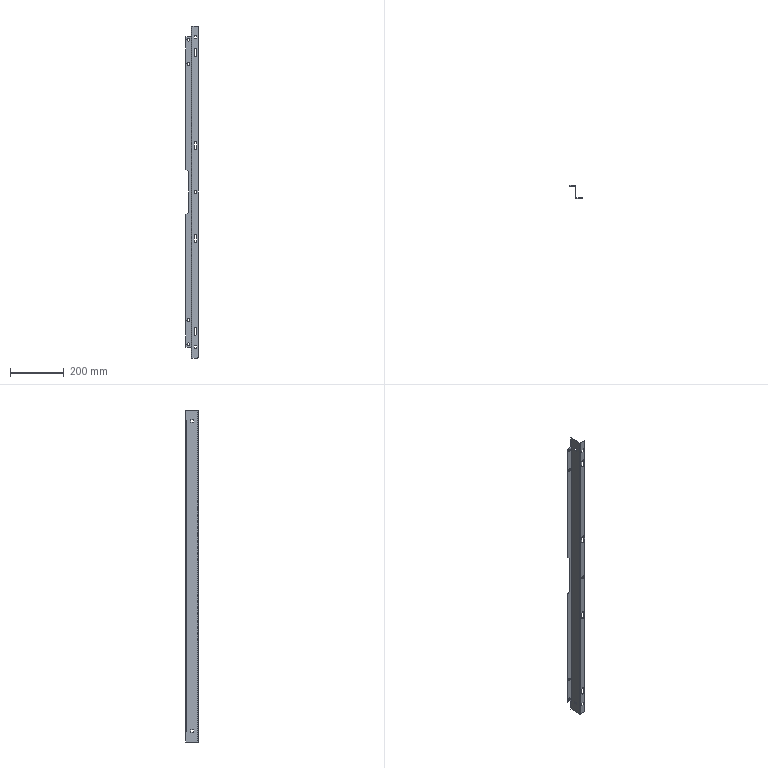Part | 1 solid | 82 faces | box 45 x 48 x 1240 mm | volume 160896 mm3 | plane 54 | cylinder 28 | commonest cylinder face diameters 10 x14 11 x8 0.4 x2 3.4 x2 4 x2